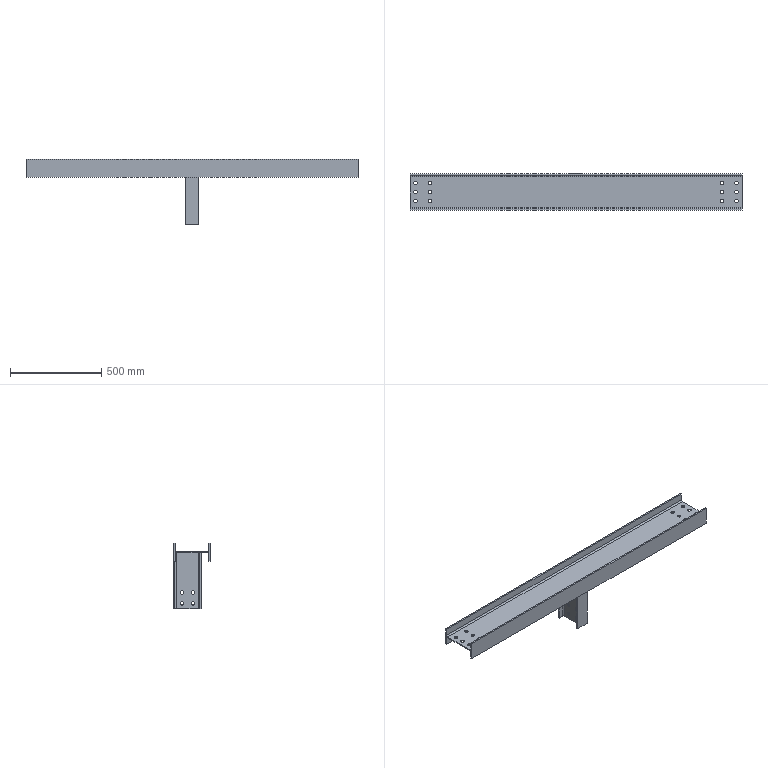Part | STEP file | 粉仓主梁12主体_Default<As Machined> | 2 solids | 71 faces | box 1815 x 200 x 360 mm | volume 5338714 mm3 | cylinder 40 | plane 31 | commonest cylinder face diameters 19 x32 16 x8